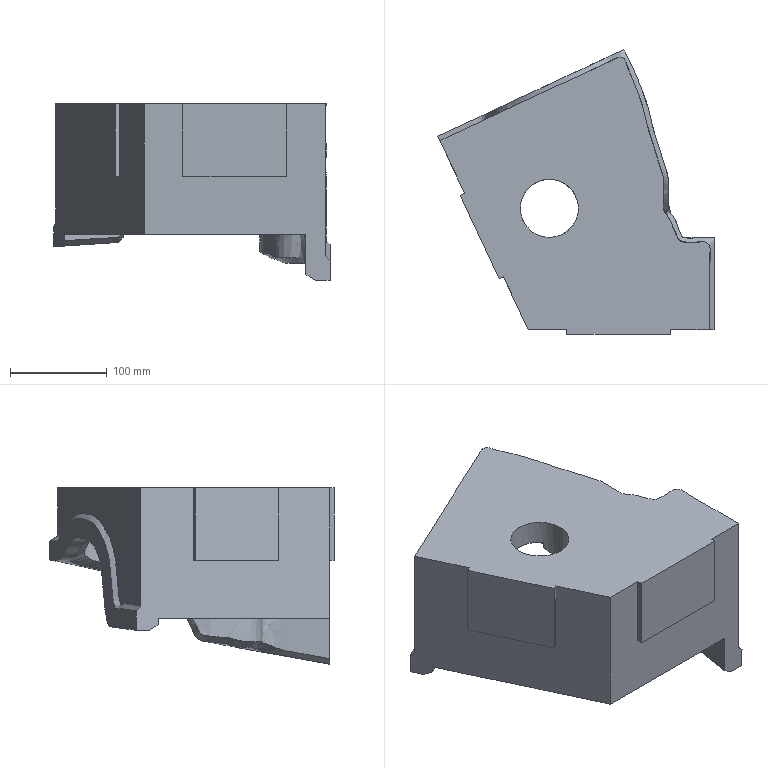Part | NX | features solid 2 | 1 solid | 41 faces | box 285 x 293.913 x 182.128 mm | volume 3390515 mm3 | plane 27 | spline 7 | cylinder 7 | commonest cylinder face diameters 30 x6 60 x1